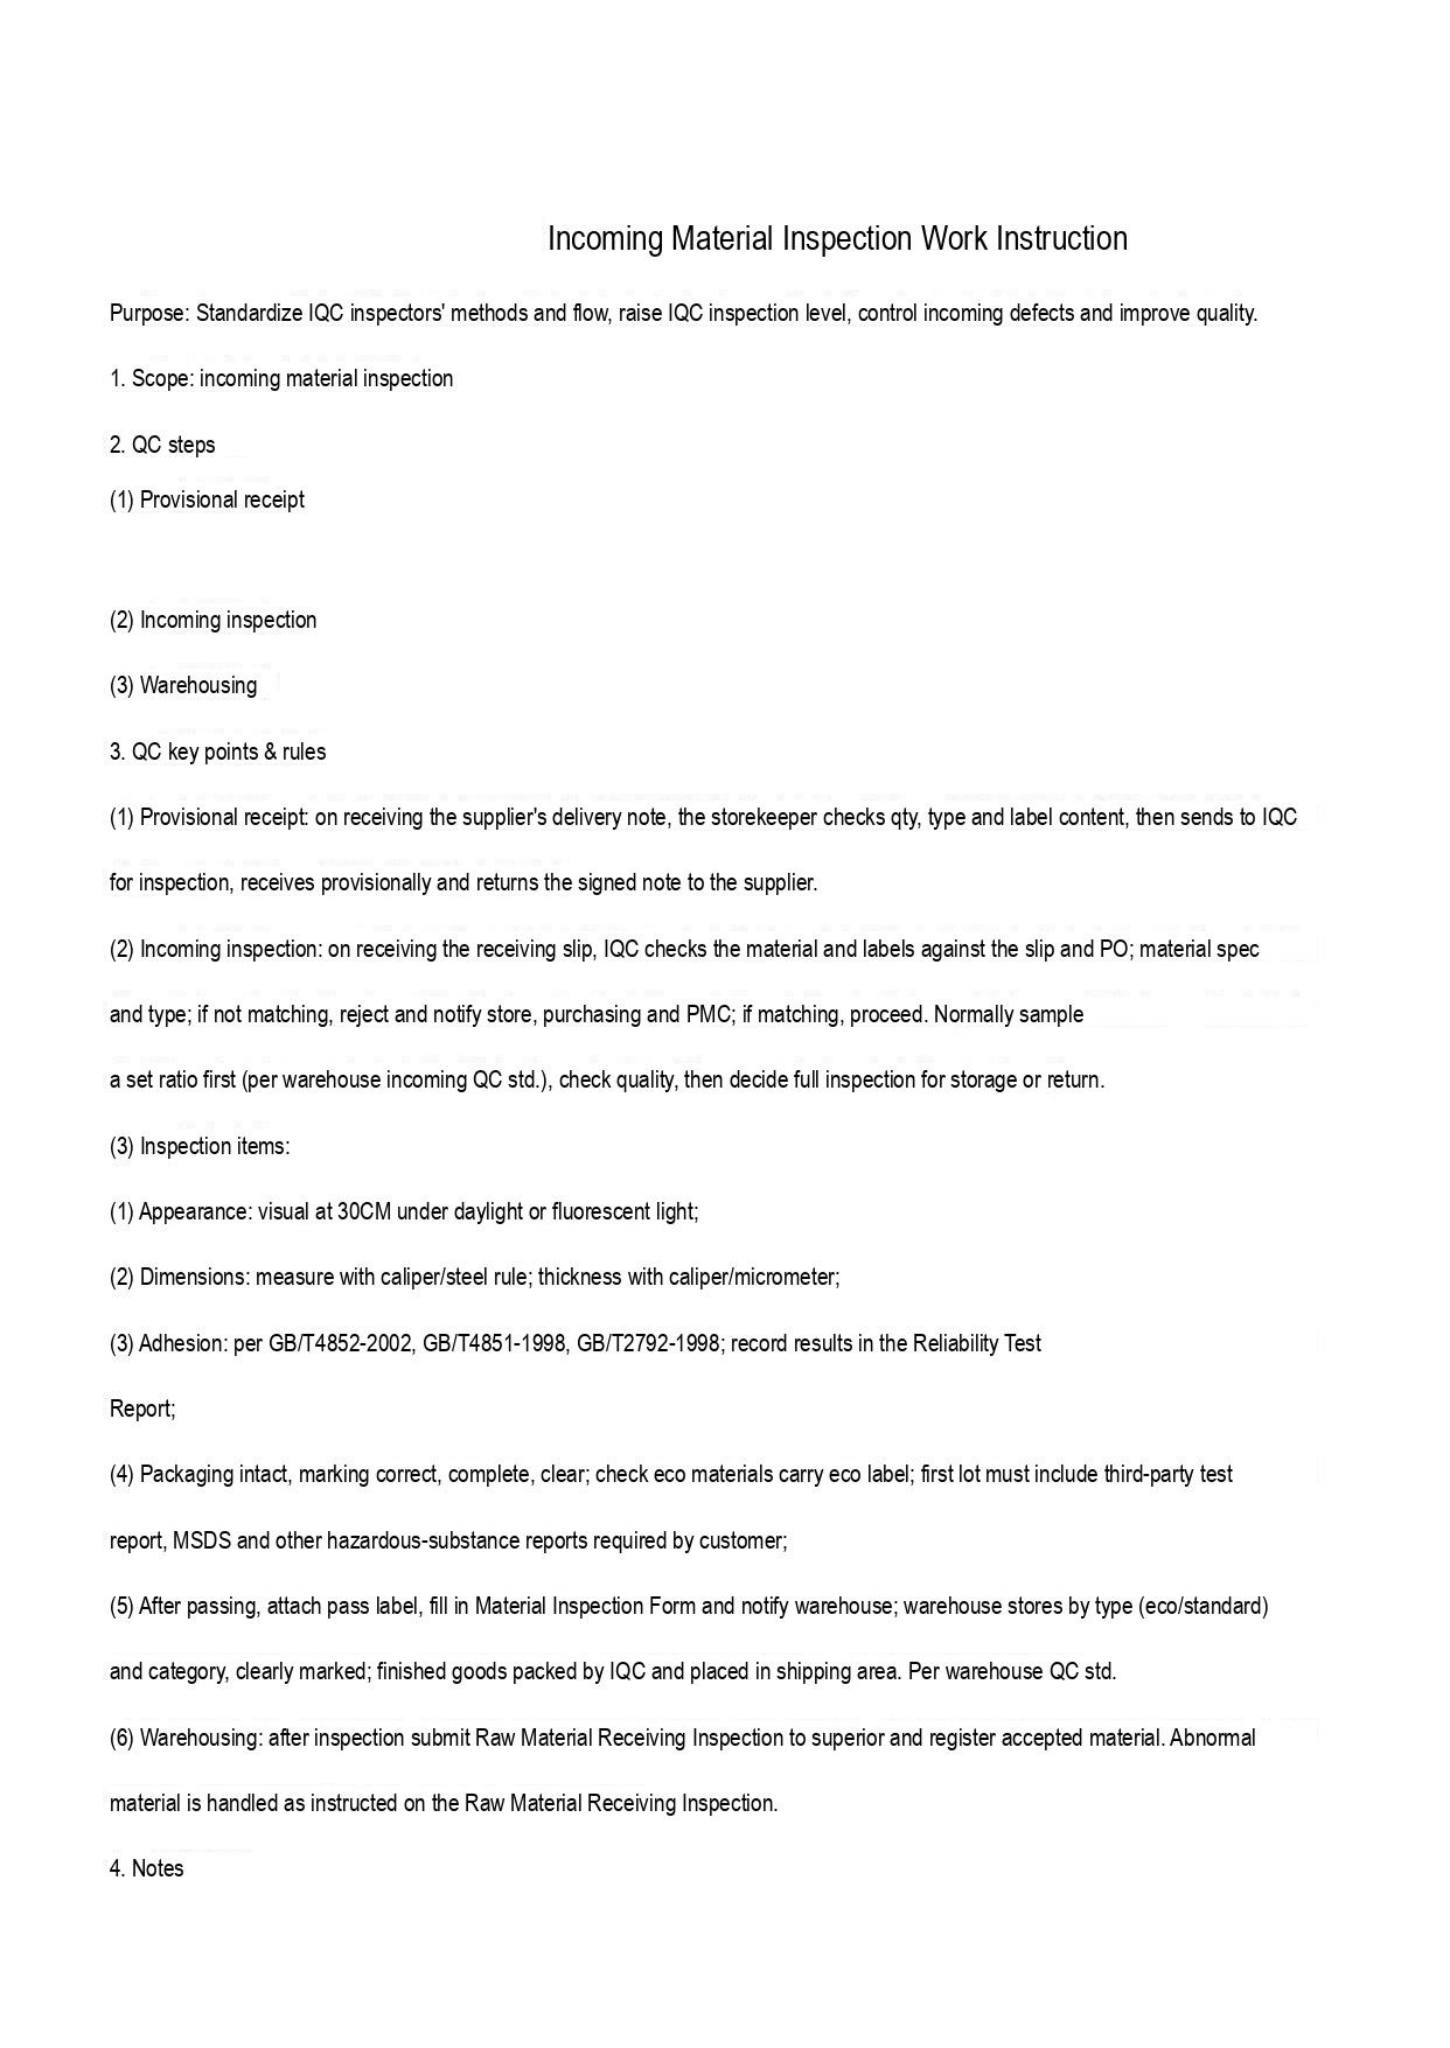Incoming Material Inspection Work Instruction

Purpose: Standardize IQC inspectors' methods and flow, raise IQC inspection level, control incoming defects and improve quality.

1. Scope: incoming material inspection

2. QC steps

(1) Provisional receipt

(2) Incoming inspection

(3) Warehousing

3. QC key points & rules

(1) Provisional receipt: on receiving the supplier's delivery note, the storekeeper checks qty, type and label content, then sends to IQC for inspection, receives provisionally and returns the signed note to the supplier.

(2) Incoming inspection: on receiving the receiving slip, IQC checks the material and labels against the slip and PO; material spec and type; if not matching, reject and notify store, purchasing and PMC; if matching, proceed. Normally sample a set ratio first (per warehouse incoming QC std.), check quality, then decide full inspection for storage or return.

(3) Inspection items:

(1) Appearance: visual at 30CM under daylight or fluorescent light;

(2) Dimensions: measure with caliper/steel rule; thickness with caliper/micrometer;

(3) Adhesion: per GB/T4852-2002, GB/T4851-1998, GB/T2792-1998; record results in the Reliability Test Report;

(4) Packaging intact, marking correct, complete, clear; check eco materials carry eco label; first lot must include third-party test report, MSDS and other hazardous-substance reports required by customer;

(5) After passing, attach pass label, fill in Material Inspection Form and notify warehouse; warehouse stores by type (eco/standard) and category, clearly marked; finished goods packed by IQC and placed in shipping area. Per warehouse QC std.

(6) Warehousing: after inspection submit Raw Material Receiving Inspection to superior and register accepted material. Abnormal material is handled as instructed on the Raw Material Receiving Inspection.

4. Notes
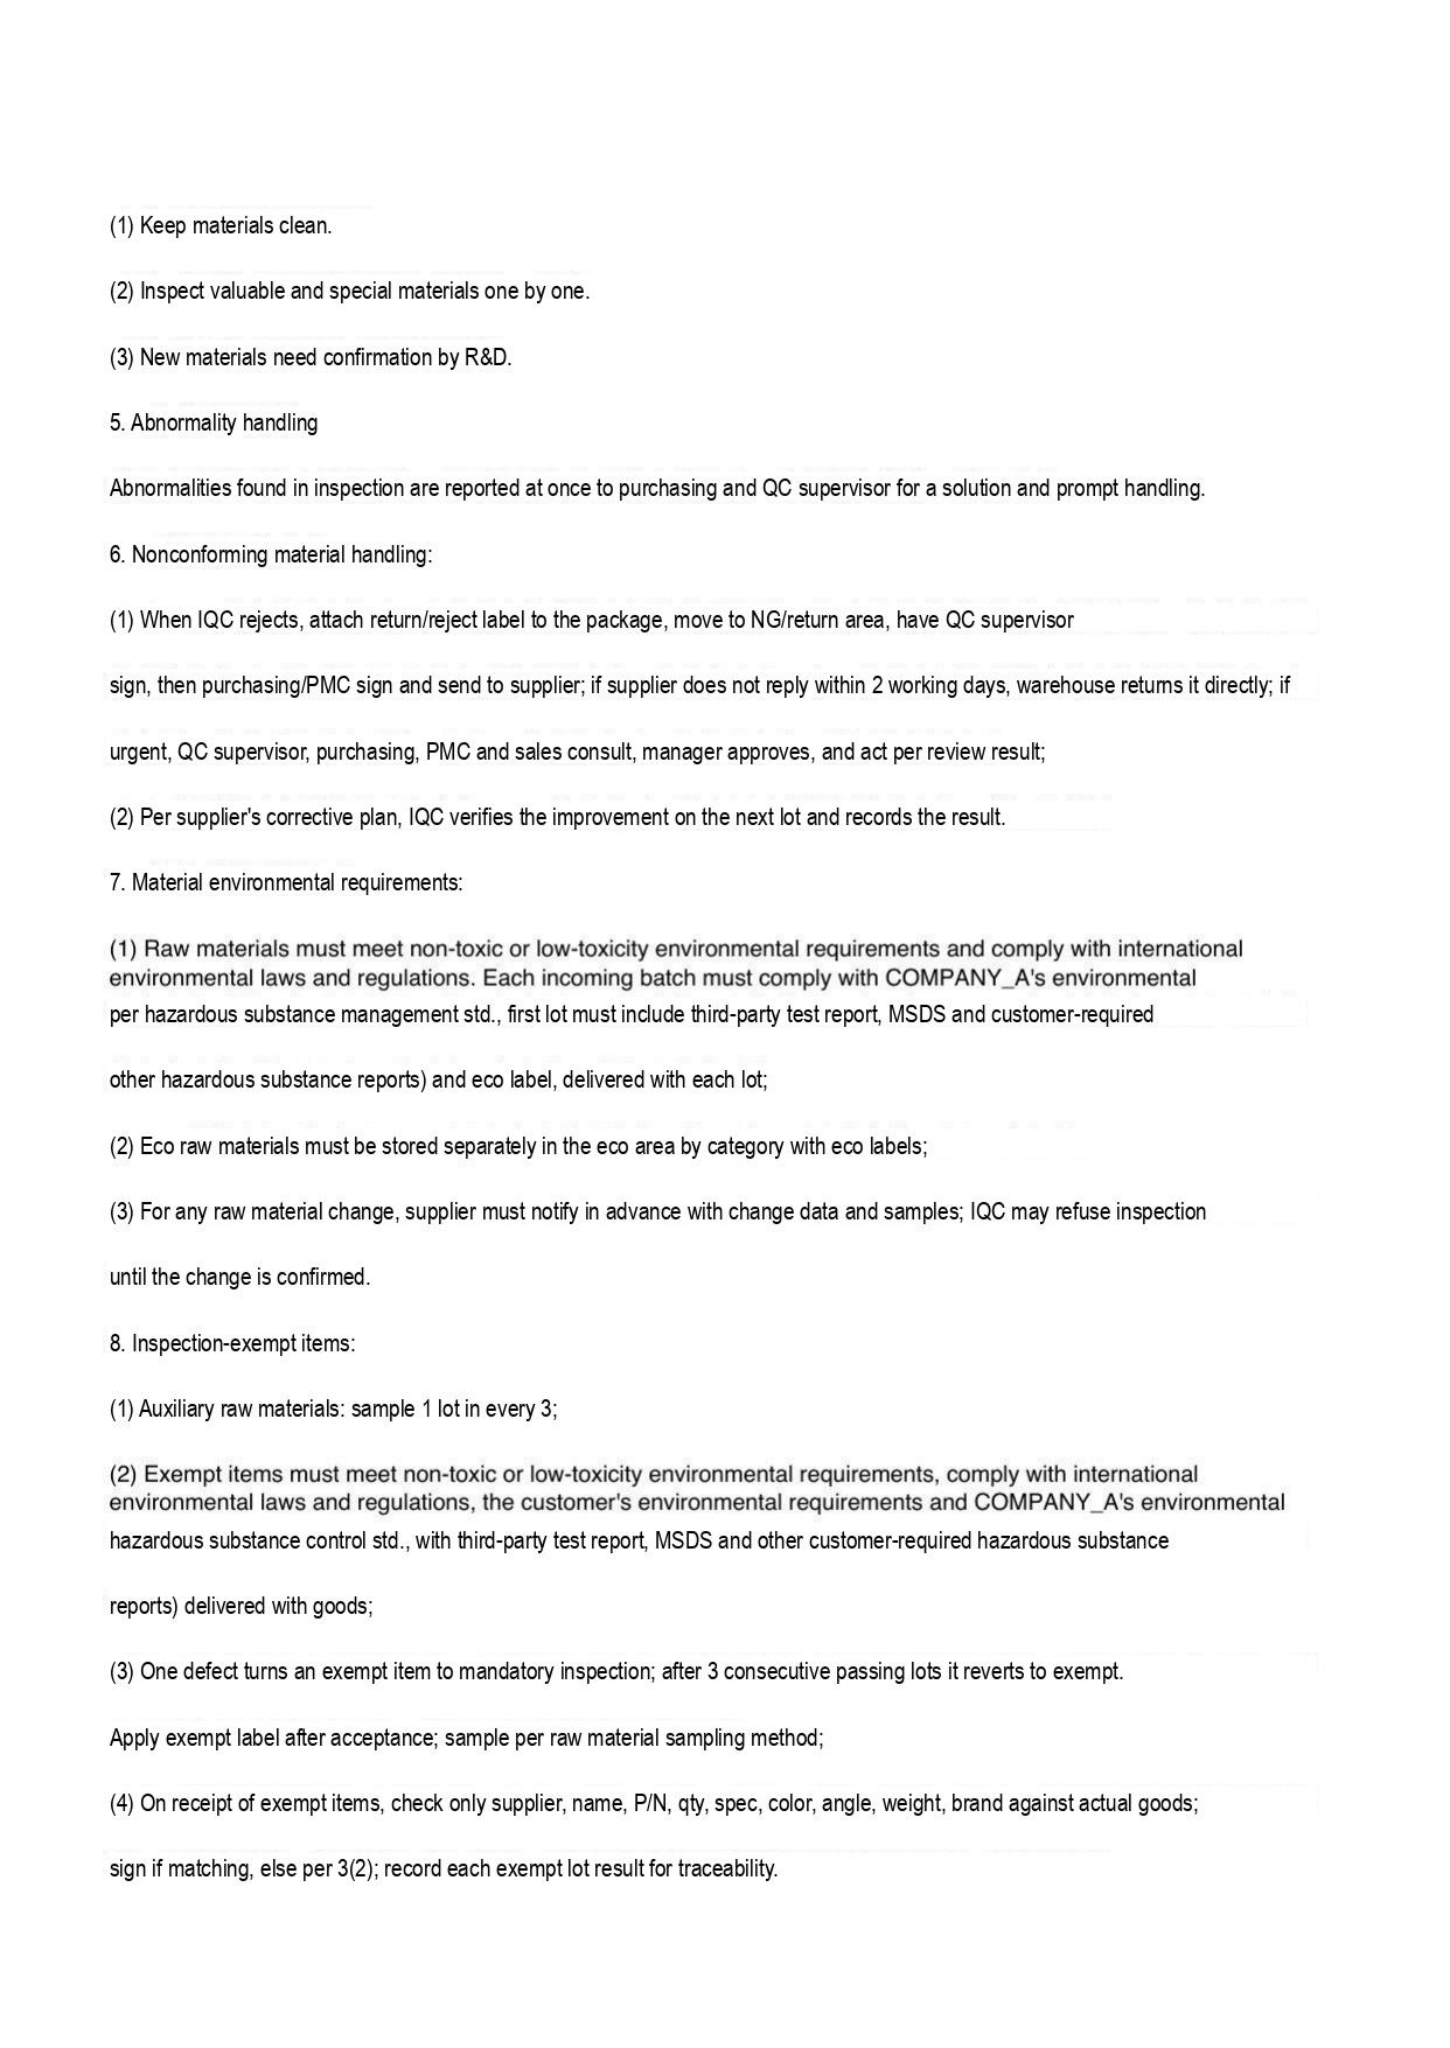(1) Keep materials clean.

(2) Inspect valuable and special materials one by one.

(3) New materials need confirmation by R&D.

5. Abnormality handling

Abnormalities found in inspection are reported at once to purchasing and QC supervisor for a solution and prompt handling.

6. Nonconforming material handling:

(1) When IQC rejects, attach return/reject label to the package, move to NG/return area, have QC supervisor

sign, then purchasing/PMC sign and send to supplier; if supplier does not reply within 2 working days, warehouse returns it directly; if

urgent, QC supervisor, purchasing, PMC and sales consult, manager approves, and act per review result;

(2) Per supplier's corrective plan, IQC verifies the improvement on the next lot and records the result.

7. Material environmental requirements:

(1) Raw materials must meet non-toxic or low-toxicity environmental requirements and comply with international environmental laws and regulations. Each incoming batch must comply with COMPANY_A's environmental
per hazardous substance management std., first lot must include third-party test report, MSDS and customer-required

other hazardous substance reports) and eco label, delivered with each lot;

(2) Eco raw materials must be stored separately in the eco area by category with eco labels;

(3) For any raw material change, supplier must notify in advance with change data and samples; IQC may refuse inspection

until the change is confirmed.

8. Inspection-exempt items:

(1) Auxiliary raw materials: sample 1 lot in every 3;

(2) Exempt items must meet non-toxic or low-toxicity environmental requirements, comply with international environmental laws and regulations, the customer's environmental requirements and COMPANY_A's environmental
hazardous substance control std., with third-party test report, MSDS and other customer-required hazardous substance

reports) delivered with goods;

(3) One defect turns an exempt item to mandatory inspection; after 3 consecutive passing lots it reverts to exempt.

Apply exempt label after acceptance; sample per raw material sampling method;

(4) On receipt of exempt items, check only supplier, name, P/N, qty, spec, color, angle, weight, brand against actual goods;

sign if matching, else per 3(2); record each exempt lot result for traceability.
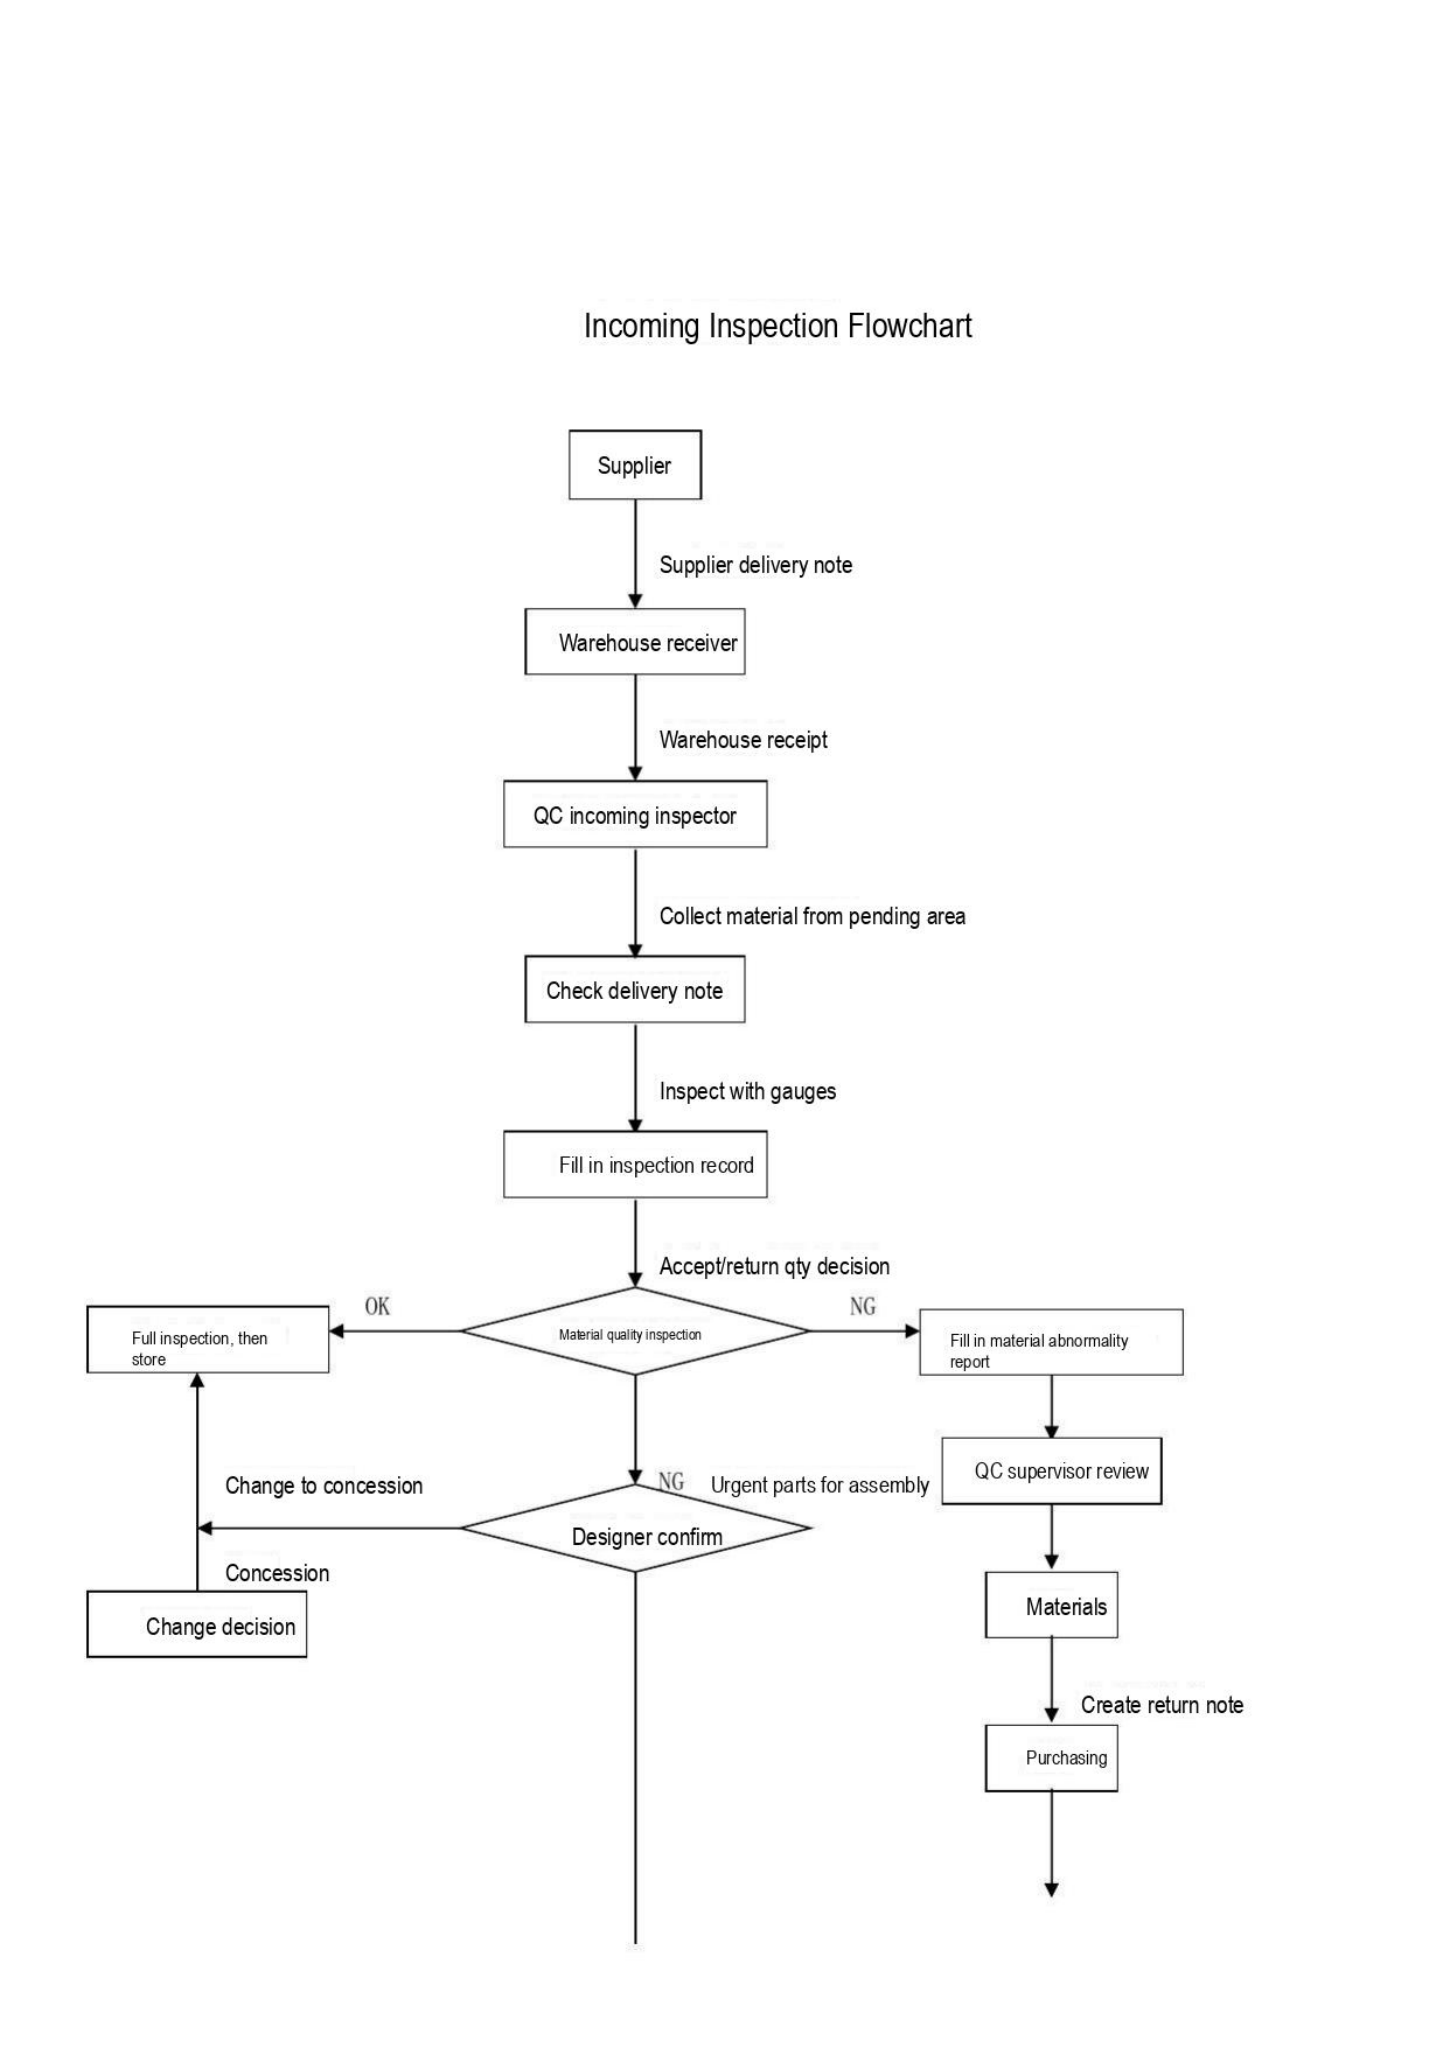Incoming Inspection Flowchart

Supplier

Supplier delivery note

Warehouse receiver

Warehouse receipt

QC incoming inspector

Collect material from pending area

Check delivery note

Inspect with gauges

Fill in inspection record

Accept/return qty decision

OK

Material quality inspection

NG

Full inspection, then store

Fill in material abnormality report

QC supervisor review

Change to concession

NG

Urgent parts for assembly

Designer confirm

Concession

Change decision

Materials

Create return note

Purchasing
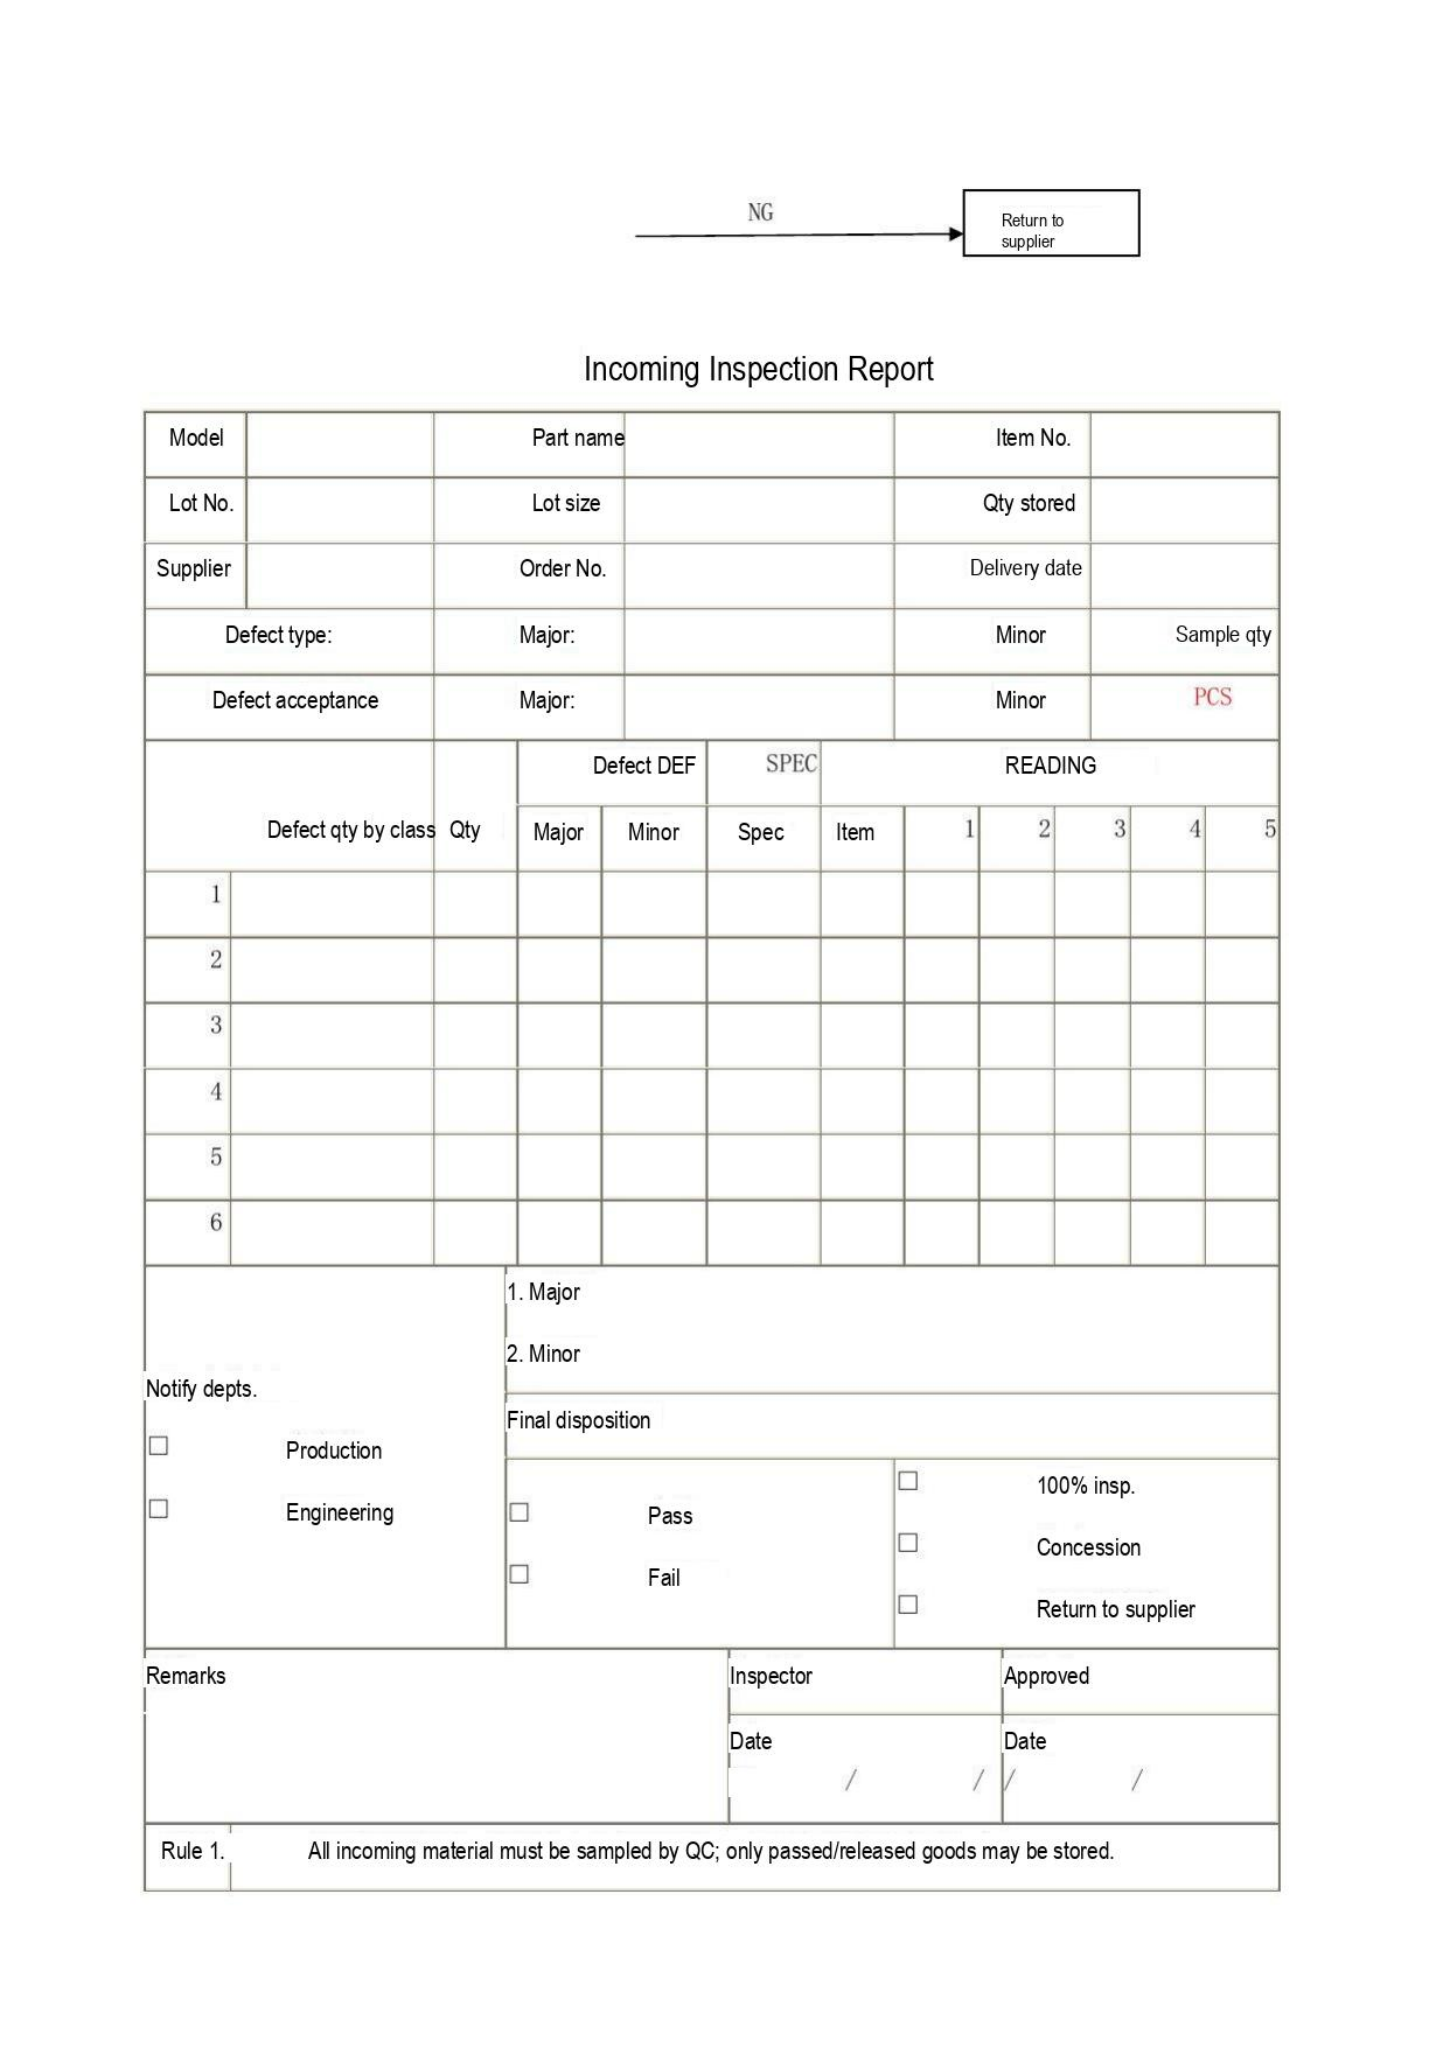NG

Return to supplier

Incoming Inspection Report

| Model | | Part name | | Item No. | |
|---|---|---|---|---|---|
| Lot No. | | Lot size | | Qty stored | |
| Supplier | | Order No. | | Delivery date | |
| Defect type: | | Major: | | Minor | Sample qty |
| Defect acceptance | | Major: | | Minor | PCS |

| | Defect qty by class | Qty | Defect DEF Major | Defect DEF Minor | SPEC Spec | READING Item | 1 | 2 | 3 | 4 | 5 |
|---|---|---|---|---|---|---|---|---|---|---|---|
| 1 | | | | | | | | | | | |
| 2 | | | | | | | | | | | |
| 3 | | | | | | | | | | | |
| 4 | | | | | | | | | | | |
| 5 | | | | | | | | | | | |
| 6 | | | | | | | | | | | |

| Notify depts. | 1. Major<br>2. Minor | |
|---|---|---|
| ☐ Production<br>☐ Engineering | Final disposition | |
| | ☐ Pass<br>☐ Fail | ☐ 100% insp.<br>☐ Concession<br>☐ Return to supplier |

| Remarks | Inspector | Approved |
|---|---|---|
| | Date / / | Date / / |

| Rule 1. | All incoming material must be sampled by QC; only passed/released goods may be stored. |
|---|---|
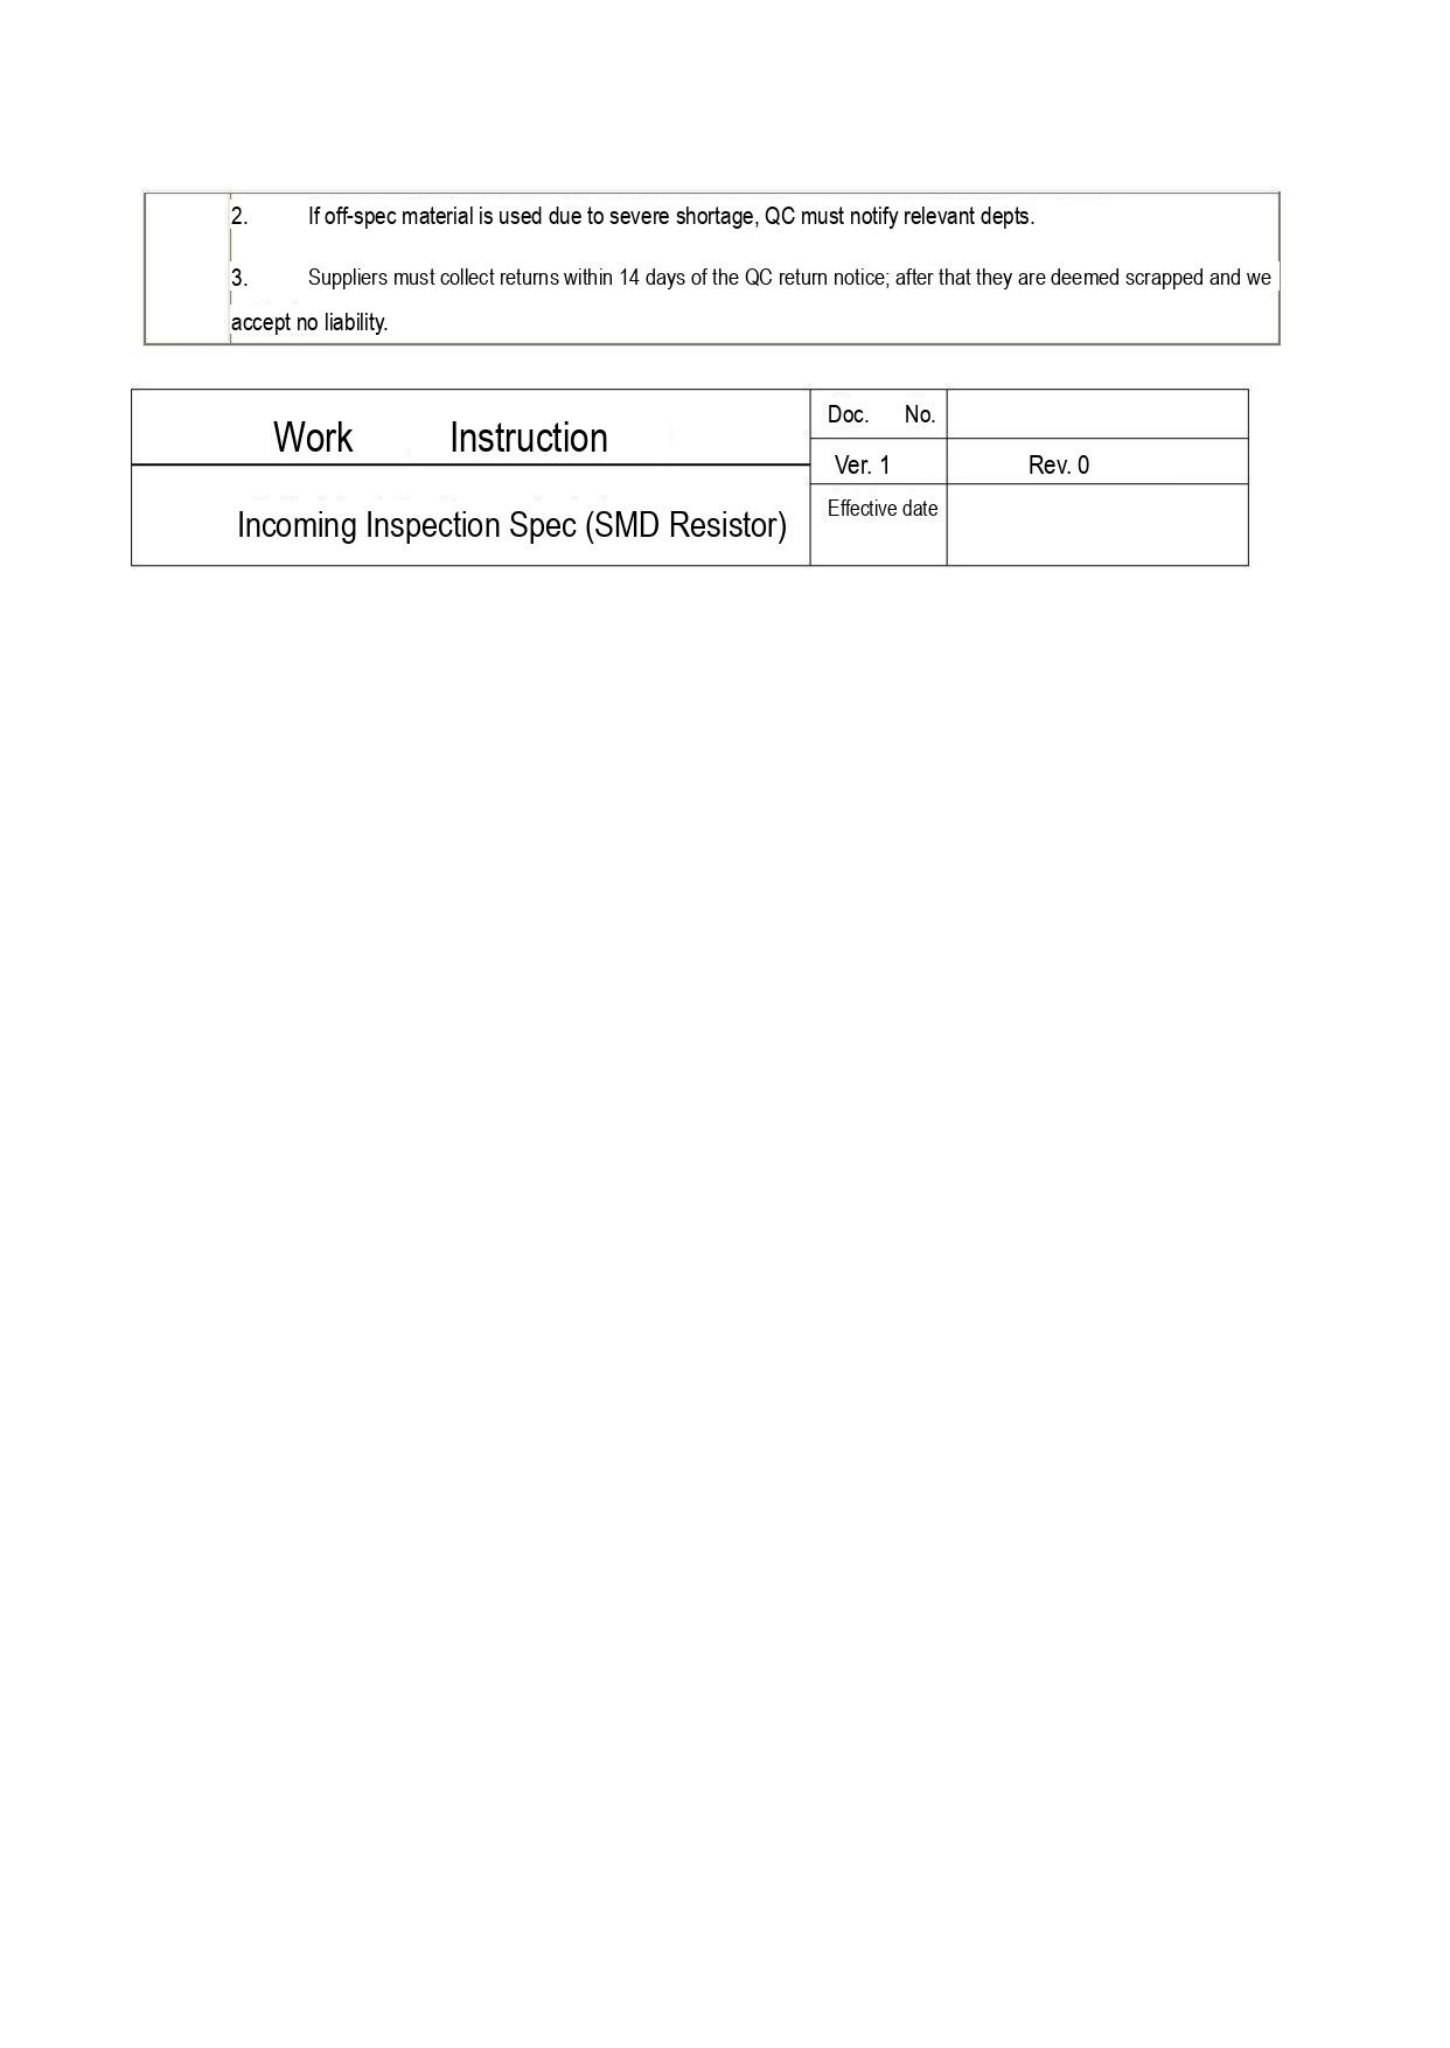| | |
|---|---|
| | 2. If off-spec material is used due to severe shortage, QC must notify relevant depts.<br>3. Suppliers must collect returns within 14 days of the QC return notice; after that they are deemed scrapped and we accept no liability. |

| Work Instruction | Doc. No. | |
|---|---|---|
| | Ver. 1 | Rev. 0 |
| Incoming Inspection Spec (SMD Resistor) | Effective date | |
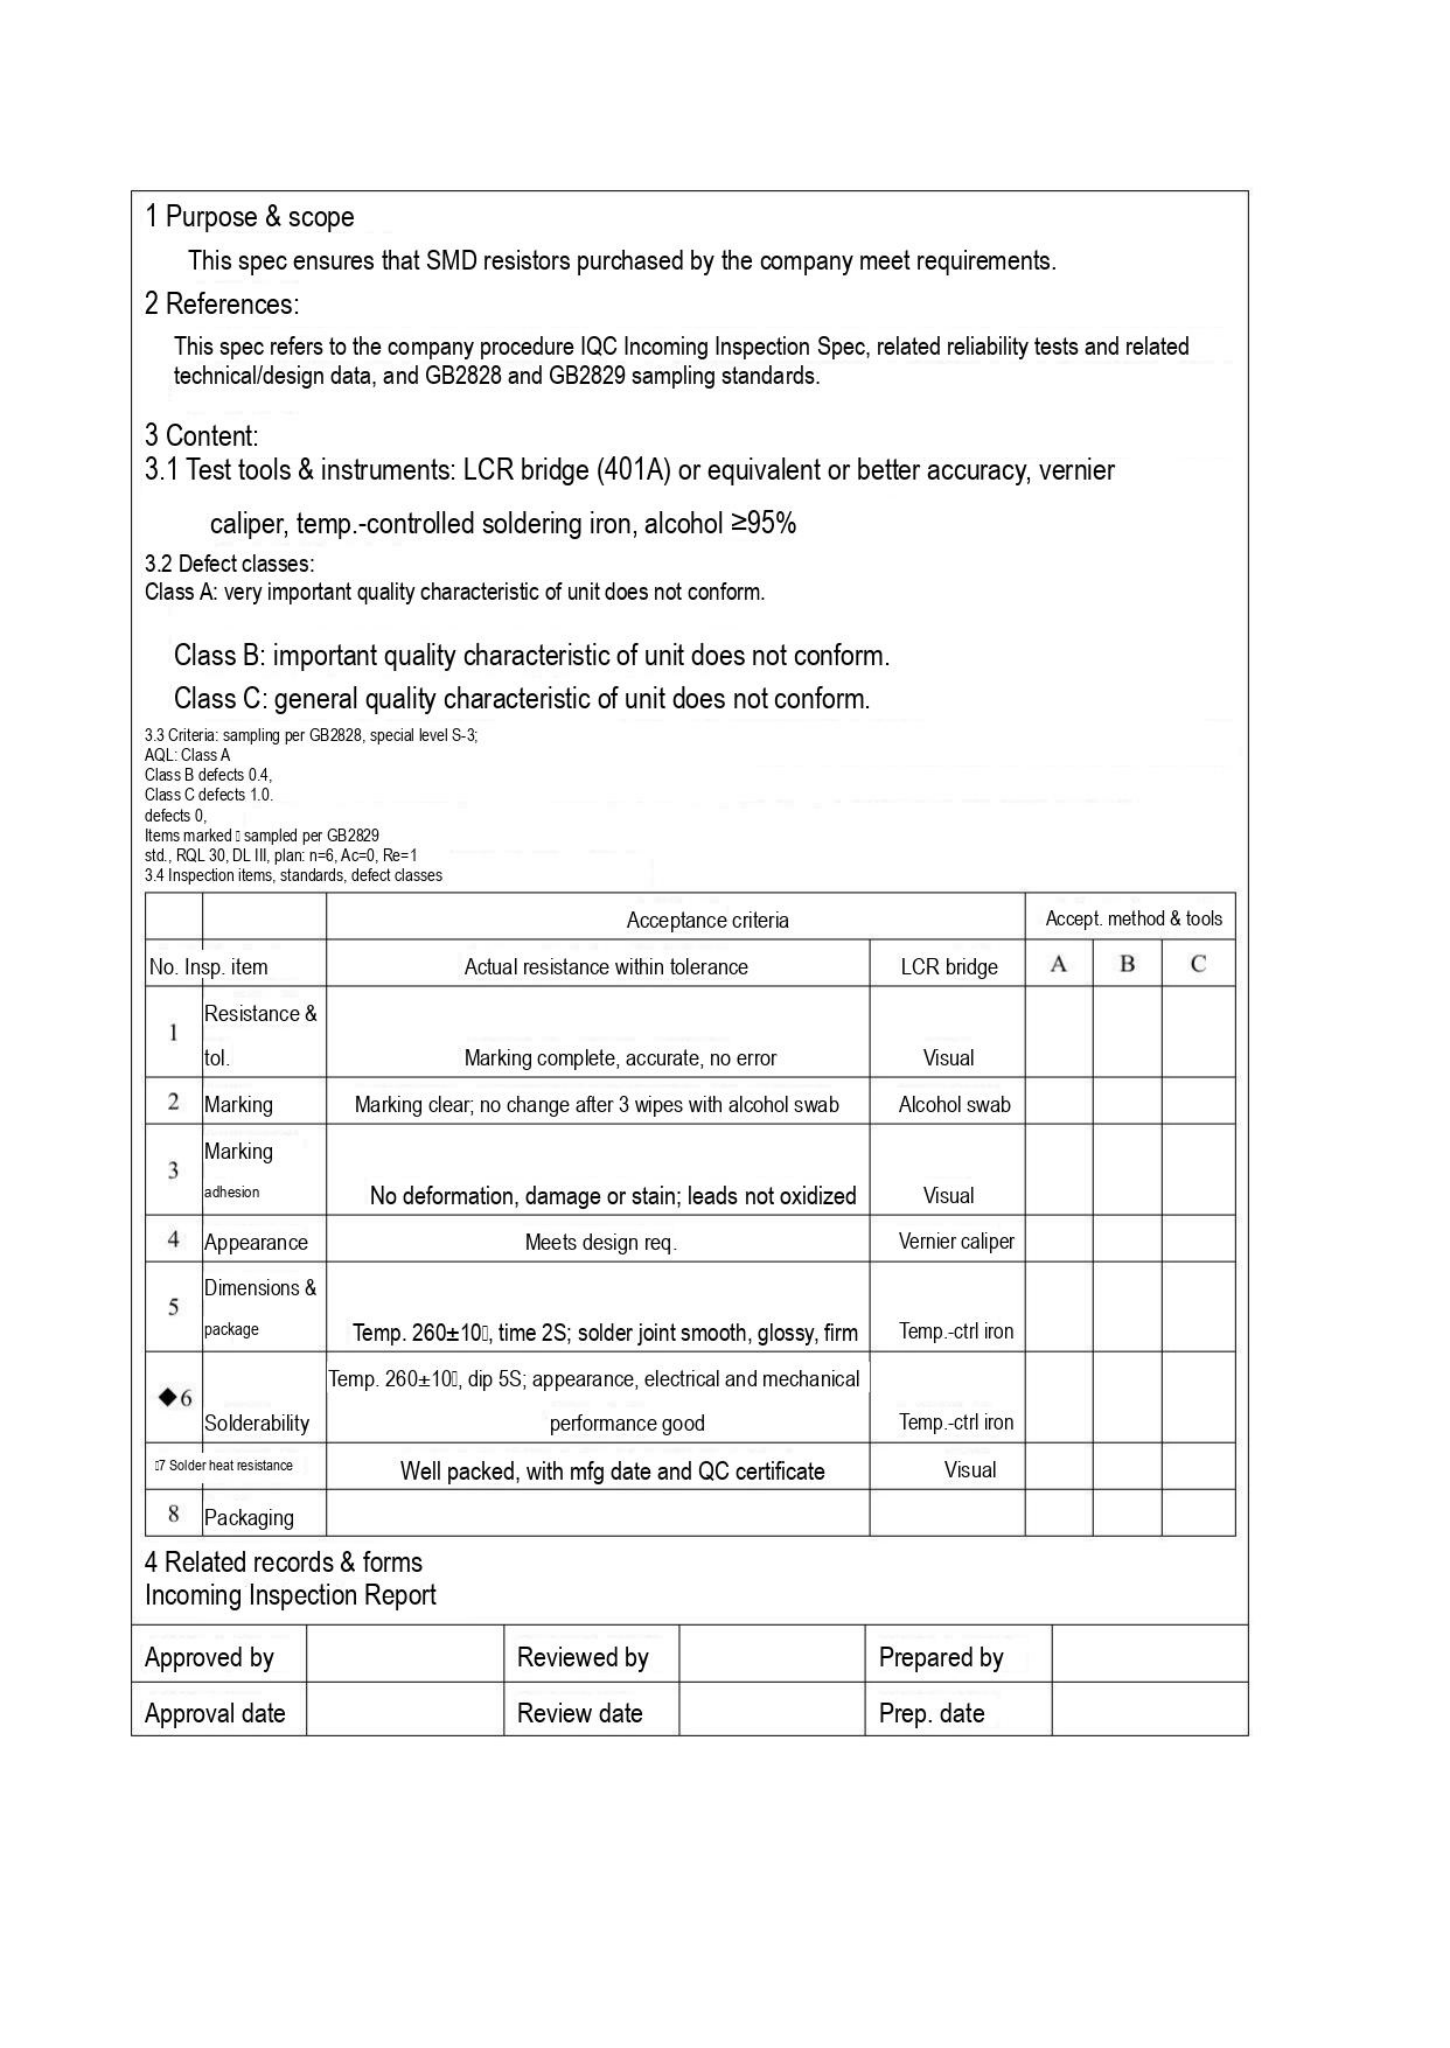1 Purpose & scope

This spec ensures that SMD resistors purchased by the company meet requirements.

2 References:

This spec refers to the company procedure IQC Incoming Inspection Spec, related reliability tests and related technical/design data, and GB2828 and GB2829 sampling standards.

3 Content:

3.1 Test tools & instruments: LCR bridge (401A) or equivalent or better accuracy, vernier caliper, temp.-controlled soldering iron, alcohol ≥95%

3.2 Defect classes:

Class A: very important quality characteristic of unit does not conform.

Class B: important quality characteristic of unit does not conform.

Class C: general quality characteristic of unit does not conform.

3.3 Criteria: sampling per GB2828, special level S-3;
AQL: Class A
Class B defects 0.4,
Class C defects 1.0.
defects 0,
Items marked sampled per GB2829
std., RQL 30, DL III, plan: n=6, Ac=0, Re=1
3.4 Inspection items, standards, defect classes

| | | Acceptance criteria | | Accept. method & tools | | |
|---|---|---|---|---|---|---|
| No. | Insp. item | Actual resistance within tolerance | LCR bridge | A | B | C |
| 1 | Resistance & tol. | Marking complete, accurate, no error | Visual | | | |
| 2 | Marking | Marking clear; no change after 3 wipes with alcohol swab | Alcohol swab | | | |
| 3 | Marking adhesion | No deformation, damage or stain; leads not oxidized | Visual | | | |
| 4 | Appearance | Meets design req. | Vernier caliper | | | |
| 5 | Dimensions & package | Temp. 260±10, time 2S; solder joint smooth, glossy, firm | Temp.-ctrl iron | | | |
| ◆6 | Solderability | Temp. 260±10, dip 5S; appearance, electrical and mechanical performance good | Temp.-ctrl iron | | | |
| 7 | Solder heat resistance | Well packed, with mfg date and QC certificate | Visual | | | |
| 8 | Packaging | | | | | |

4 Related records & forms
Incoming Inspection Report

| Approved by | | Reviewed by | | Prepared by | |
|---|---|---|---|---|---|
| Approval date | | Review date | | Prep. date | |
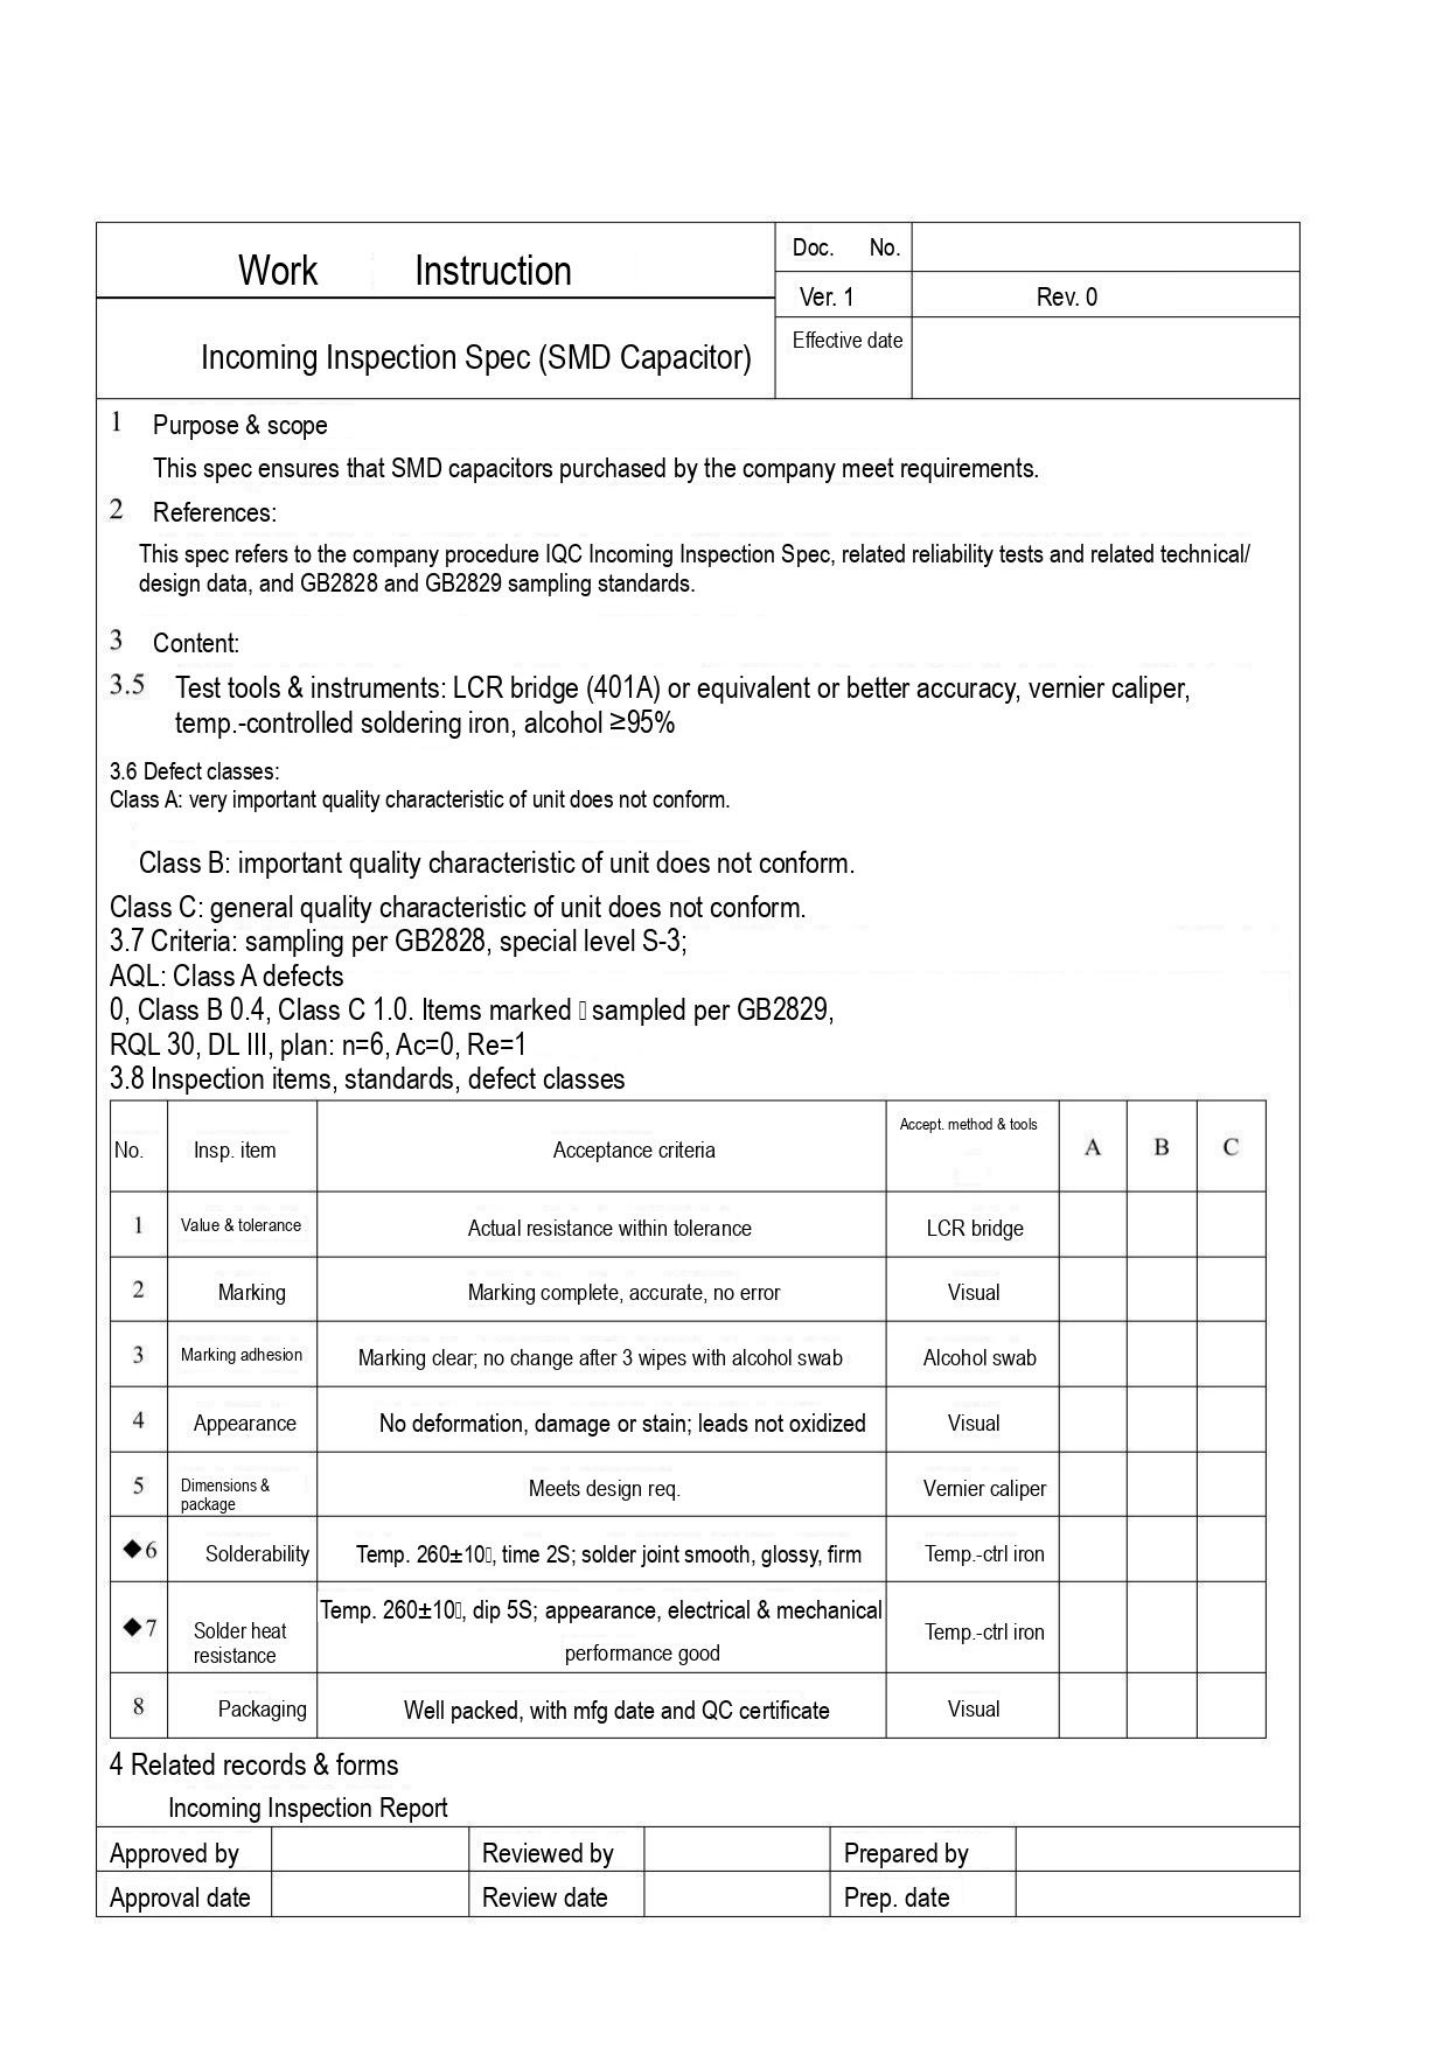# Work Instruction

| Doc. No. | |
|---|---|
| Ver. 1 | Rev. 0 |
| Effective date | |

Incoming Inspection Spec (SMD Capacitor)

1 Purpose & scope

This spec ensures that SMD capacitors purchased by the company meet requirements.

2 References:

This spec refers to the company procedure IQC Incoming Inspection Spec, related reliability tests and related technical/ design data, and GB2828 and GB2829 sampling standards.

3 Content:

3.5 Test tools & instruments: LCR bridge (401A) or equivalent or better accuracy, vernier caliper, temp.-controlled soldering iron, alcohol ≥95%

3.6 Defect classes:
Class A: very important quality characteristic of unit does not conform.

Class B: important quality characteristic of unit does not conform.

Class C: general quality characteristic of unit does not conform.
3.7 Criteria: sampling per GB2828, special level S-3;
AQL: Class A defects
0, Class B 0.4, Class C 1.0. Items marked □ sampled per GB2829,
RQL 30, DL III, plan: n=6, Ac=0, Re=1
3.8 Inspection items, standards, defect classes

| No. | Insp. item | Acceptance criteria | Accept. method & tools | A | B | C |
|---|---|---|---|---|---|---|
| 1 | Value & tolerance | Actual resistance within tolerance | LCR bridge | | | |
| 2 | Marking | Marking complete, accurate, no error | Visual | | | |
| 3 | Marking adhesion | Marking clear; no change after 3 wipes with alcohol swab | Alcohol swab | | | |
| 4 | Appearance | No deformation, damage or stain; leads not oxidized | Visual | | | |
| 5 | Dimensions & package | Meets design req. | Vernier caliper | | | |
| ◆6 | Solderability | Temp. 260±10□, time 2S; solder joint smooth, glossy, firm | Temp.-ctrl iron | | | |
| ◆7 | Solder heat resistance | Temp. 260±10□, dip 5S; appearance, electrical & mechanical performance good | Temp.-ctrl iron | | | |
| 8 | Packaging | Well packed, with mfg date and QC certificate | Visual | | | |

4 Related records & forms

Incoming Inspection Report

| Approved by | | Reviewed by | | Prepared by | |
|---|---|---|---|---|---|
| Approval date | | Review date | | Prep. date | |